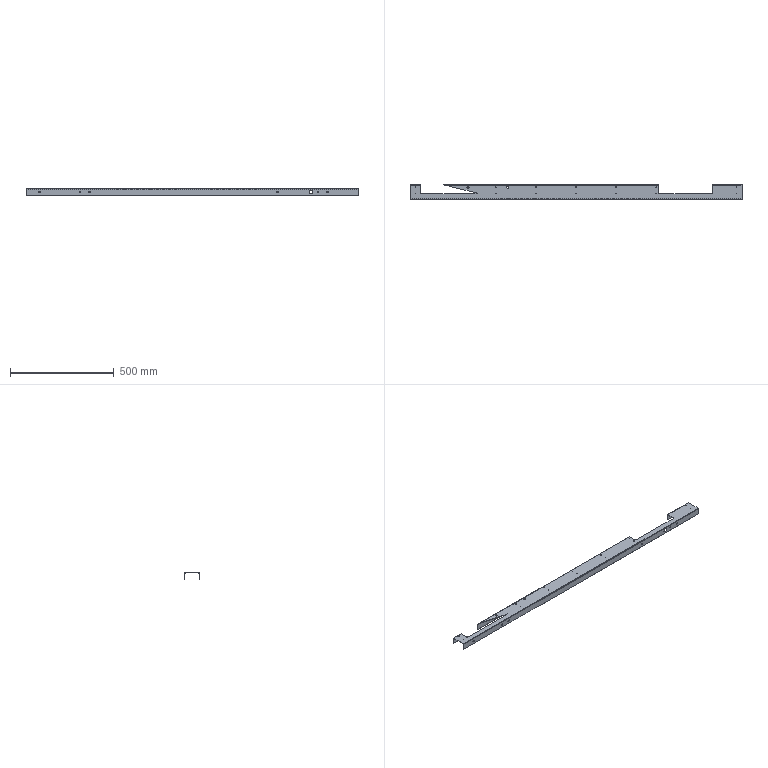Part | SolidWorks | features Cut 6, EdgeFlange 1, Fillet 1, FlatPattern 1, SMBaseFlange 1, SheetMetal 1 | 1 solid | 97 faces | box 1598 x 70 x 32 mm | volume 211642 mm3 | cylinder 58 | plane 39 | commonest cylinder face diameters 3 x28 10 x8 2.4 x4 4.8 x4 5.5 x4 5.371 x2